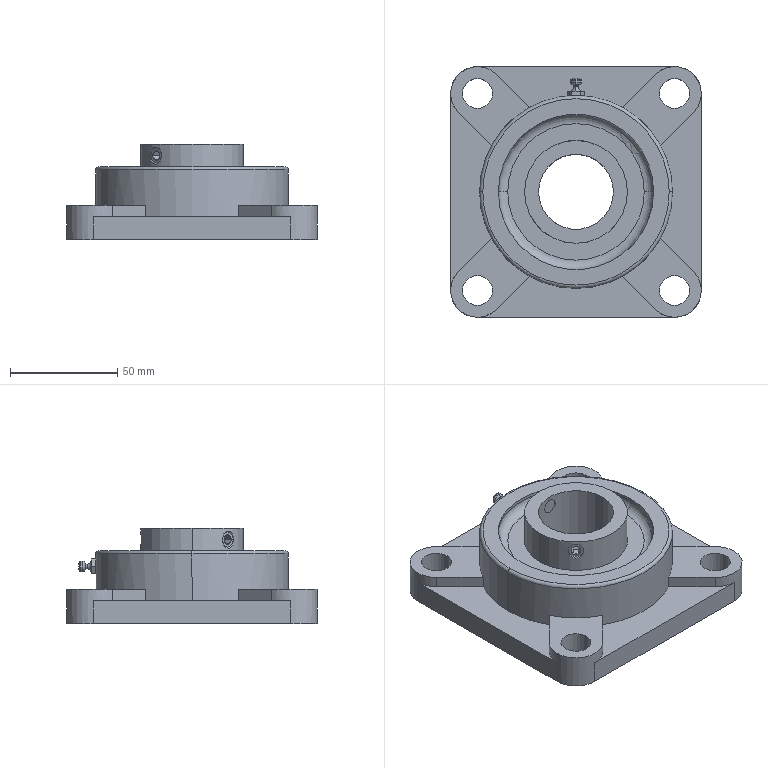Part | STEP file | PN_0050_square pillow block bearing | 3 solids | 149 faces | box 117 x 117 x 44.4 mm | volume 243973 mm3 | plane 62 | cylinder 38 | cone 31 | torus 16 | spline 2 | commonest cylinder face diameters 14 x8 25 x6 6.917 x4 8 x4 48 x4 72.5 x4